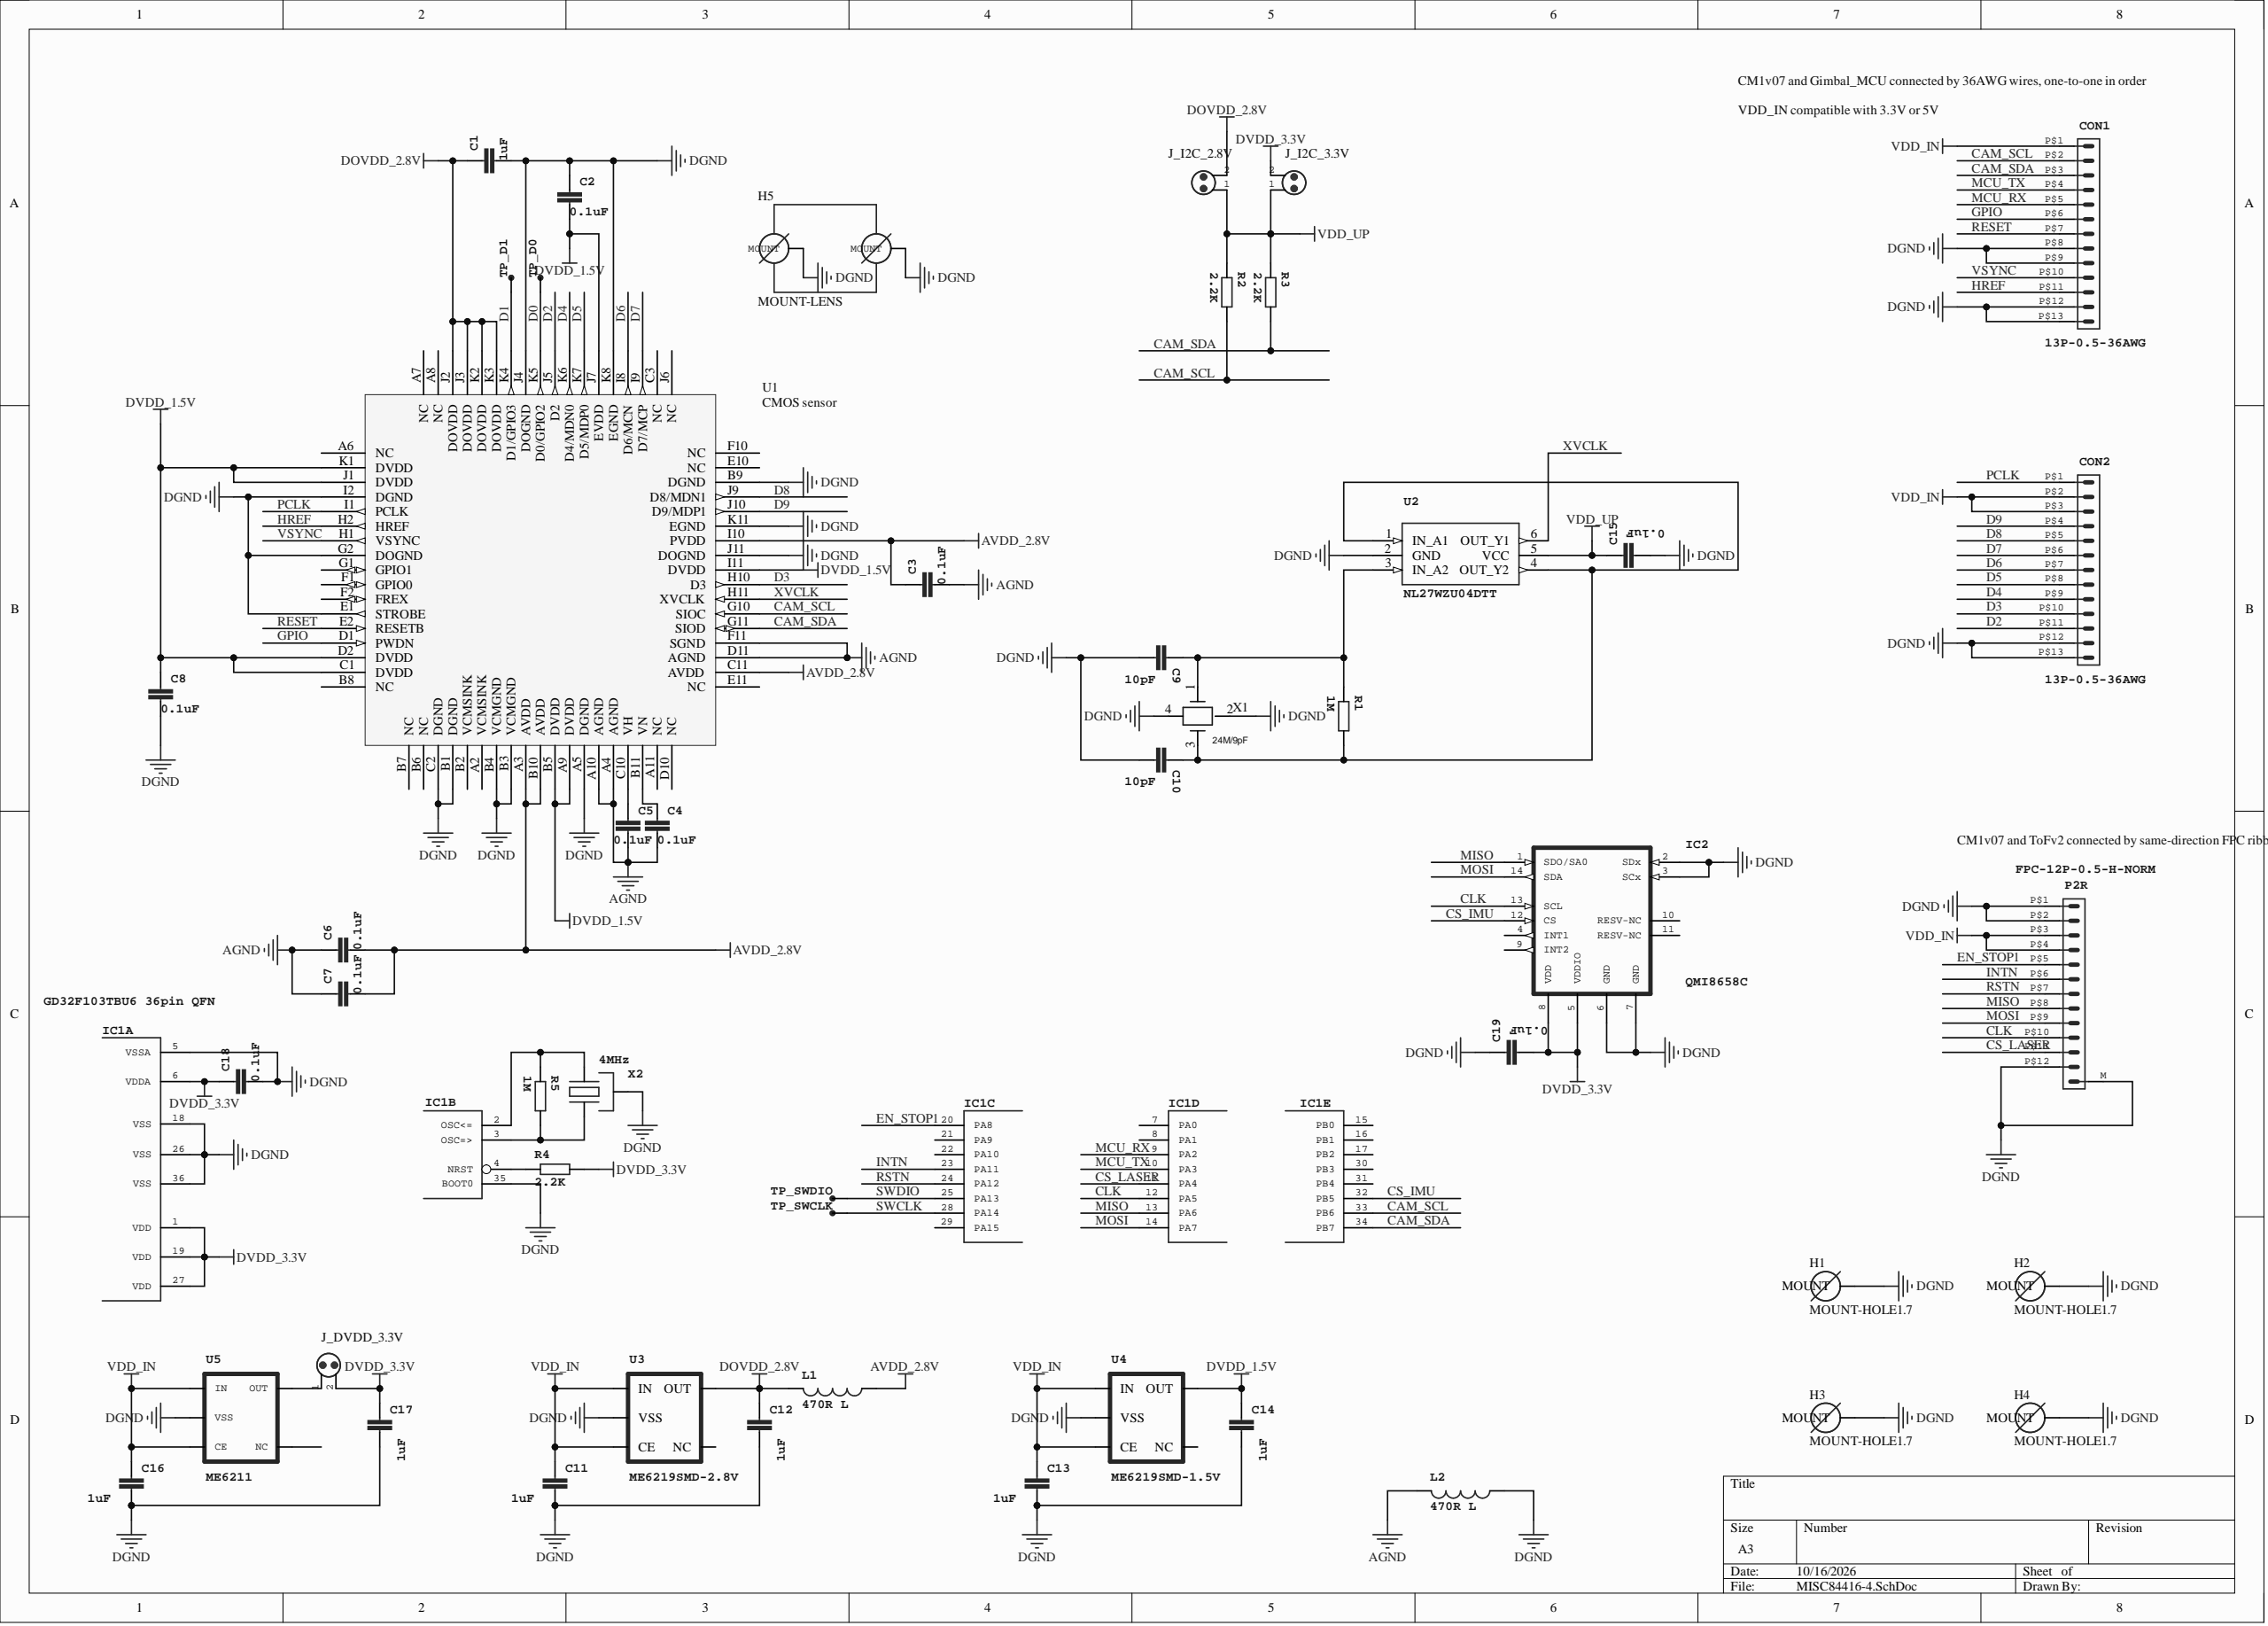Circuit board | Altium Designer | 50 parts | 46 nets
Bill of materials:
Comment,Description,Designator,Footprint,LibRef,Quantity
"1uF","","C1, C11, C12, C13, C14, C16, C17","RCL_C0402_TI","RCL_C-EUC0402_TI","7"
"0.1uF","","C2, C3, C4, C5, C6, C7, C8, C15, C18, C19","RCL_C0402_TI","RCL_C-EUC0402_TI","10"
"10pF","","C9, C10","RCL_C0402_TI","RCL_C-EUC0402_TI","2"
"13P-0.5-36AWG","","CON1, CON2","13P-0.5-36AWG","13P-0.5-36AWG","2"
"MOUNT-HOLE1.7","","H1, H2, H3, H4","MOUNT-HOLE1.7","MOUNT-HOLE1.7","4"
"MOUNT-LENS","","H5","MOUNT-LENS-M12-1.6","MOUNT-LENS","1"
"GD32F103TBU6 36pin QFN","","IC1","GD32_QFN36","GD32F103TBU6","1"
"QMI8658C","","IC2","LGA14_3X2.5","QMI8658C","1"
"JUMPER_2P_MIN","","J_DVDD_3.3V, J_I2C_2.8V, J_I2C_3.3V","JUMPER_2P_MIN","JUMPER_2P_MIN","3"
"470R L","","L1, L2","RCL_L0603","RCL_L-USL0603","2"
"FPC-12P-0.5-H-NORM","","P2R","FPC-12P-0.5-H-NORM","FPC-12P-0.5-H-NORM","1"
"1M","","R1, R5","RCL_R0402_TI","RCL_R-EUR0402_TI","2"
"2.2K","","R2, R3, R4","RCL_R0402_TI","RCL_R-EUR0402_TI","3"
"","","TP_D0, TP_D1, TP_SWCLK, TP_SWDIO","TP-1","TP-1","4"
"CMOS sensor","1/4INCH","U1","BGA71_5.99X5.84","OV5640","1"
"NL27WZU04DTT","","U2","SOT23-6","NL27WZU04DTT","1"
"ME6219SMD-2.8V","","U3","SOT23-5","ME6219SMD","1"
"ME6219SMD-1.5V","","U4","SOT23-5","ME6219SMD","1"
"ME6211","","U5","SOT23-5","ME6211SMD","1"
"24M/9pF","","X1","EPSON-TSX3225","XTAL_EPSON_3225","1"
"4MHz","","X2","XTAL_4.5X2.0","XTAL_MURATA-4.5X2.0","1"
Netlist (Protel format):
[
C1
RCL_C0402_TI
1uF



]
[
C2
RCL_C0402_TI
0.1uF



]
[
C3
RCL_C0402_TI
0.1uF



]
[
C4
RCL_C0402_TI
0.1uF



]
[
C5
RCL_C0402_TI
0.1uF



]
[
C6
RCL_C0402_TI
0.1uF



]
[
C7
RCL_C0402_TI
0.1uF



]
[
C8
RCL_C0402_TI
0.1uF



]
[
C9
RCL_C0402_TI
10pF



]
[
C10
RCL_C0402_TI
10pF



]
[
C11
RCL_C0402_TI
1uF



]
[
C12
RCL_C0402_TI
1uF



]
[
C13
RCL_C0402_TI
1uF



]
[
C14
RCL_C0402_TI
1uF



]
[
C15
RCL_C0402_TI
0.1uF



]
[
C16
RCL_C0402_TI
1uF



]
[
C17
RCL_C0402_TI
1uF



]
[
C18
RCL_C0402_TI
0.1uF



]
[
C19
RCL_C0402_TI
0.1uF



]
[
CON1
13P-0.5-36AWG
13P-0.5-36AWG



]
[
CON2
13P-0.5-36AWG
13P-0.5-36AWG



]
[
H1
MOUNT-HOLE1.7
MOUNT-HOLE1.7



]
[
H2
MOUNT-HOLE1.7
MOUNT-HOLE1.7



]
[
H3
MOUNT-HOLE1.7
MOUNT-HOLE1.7



]
[
H4
MOUNT-HOLE1.7
MOUNT-HOLE1.7



]
[
H5
MOUNT-LENS-M12-1.6
MOUNT-LENS



]
[
IC1
GD32_QFN36
GD32F103TBU6 36pin QFN



]
[
IC2
LGA14_3X2.5
QMI8658C



]
[
J_DVDD_3.3V
JUMPER_2P_MIN
JUMPER_2P_MIN



]
[
J_I2C_2.8V
JUMPER_2P_MIN
JUMPER_2P_MIN



]
[
J_I2C_3.3V
JUMPER_2P_MIN
JUMPER_2P_MIN



]
[
L1
RCL_L0603
470R L



]
[
L2
RCL_L0603
470R L



]
[
P2R
FPC-12P-0.5-H-NORM
FPC-12P-0.5-H-NORM



]
[
R1
RCL_R0402_TI
1M



]
[
R2
RCL_R0402_TI
2.2K



]
[
R3
RCL_R0402_TI
2.2K



]
[
R4
RCL_R0402_TI
2.2K



]
[
R5
RCL_R0402_TI
1M



]
[
TP_D0
TP-1




]
[
TP_D1
TP-1




]
[
TP_SWCLK
TP-1




]
[
TP_SWDIO
TP-1




]
[
U1
BGA71_5.99X5.84
CMOS sensor



]
[
U2
SOT23-6
NL27WZU04DTT



]
[
U3
SOT23-5
ME6219SMD-2.8V



]
[
U4
SOT23-5
ME6219SMD-1.5V



]
[
U5
SOT23-5
ME6211



]
[
X1
EPSON-TSX3225
24M/9pF



]
[
X2
XTAL_4.5X2.0
4MHz



]
(
XVCLK
U1-H11
U2-6
)
(
VSYNC
CON1-P$10
U1-H1
)
(
VDD_UP
C15-1
J_I2C_2.8V-1
J_I2C_3.3V-1
R2-1
R3-1
U2-5
)
(
VDD_IN
C11-1
C13-1
C16-1
CON1-P$1
CON2-P$2
CON2-P$3
P2R-P$3
P2R-P$4
U3-1
U3-3
U4-1
U4-3
U5-1
U5-3
)
(
SWDIO
IC1-25
TP_SWDIO-1
)
(
SWCLK
IC1-28
TP_SWCLK-1
)
(
RSTN
IC1-24
P2R-P$7
)
(
RESET
CON1-P$7
U1-E2
)
(
PCLK
CON2-P$1
U1-I1
)
(
NetJ_DVDD_3.3V_1
J_DVDD_3.3V-1
U5-5
)
(
NetIC1_4
IC1-4
R4-1
)
(
NetIC1_3
IC1-3
R5-2
X2-1
)
(
NetIC1_2
IC1-2
R5-1
X2-3
)
(
NetC10_1
C10-1
R1-2
U2-1
U2-4
X1-3
)
(
NetC9_1
C9-1
R1-1
U2-3
X1-1
)
(
NetC5_1
C5-1
U1-C10
)
(
NetC4_1
C4-1
U1-B11
)
(
MOSI
IC1-14
IC2-14
P2R-P$9
)
(
MISO
IC1-13
IC2-1
P2R-P$8
)
(
MCU_TX
CON1-P$4
IC1-10
)
(
MCU_RX
CON1-P$5
IC1-9
)
(
INTN
IC1-23
P2R-P$6
)
(
HREF
CON1-P$11
U1-H2
)
(
GPIO
CON1-P$6
U1-D1
)
(
EN_STOP1
IC1-20
P2R-P$5
)
(
DVDD_3.3V
C17-1
C18-1
C19-2
IC1-1
IC1-6
IC1-19
IC1-27
IC2-5
IC2-8
J_DVDD_3.3V-2
J_I2C_3.3V-2
R4-2
)
(
DVDD_1.5V
C2-2
C8-1
C14-1
U1-A9
U1-B5
U1-C1
U1-D2
U1-I11
U1-J1
U1-J7
U1-K1
U4-5
)
(
DOVDD_2.8V
C1-1
C12-1
J_I2C_2.8V-2
L1-2
U1-J2
U1-J3
U1-K2
U1-K3
U3-5
)
(
DGND
C1-2
C2-1
C8-2
C9-2
C10-2
C11-2
C12-2
C13-2
C14-2
C15-2
C16-2
C17-2
C18-2
C19-1
CON1-P$8
CON1-P$9
CON1-P$12
CON1-P$13
CON2-P$12
CON2-P$13
H1-MOUNT
H2-MOUNT
H3-MOUNT
H4-MOUNT
H5-MOUNT
IC1-5
IC1-18
IC1-26
IC1-35
IC1-36
IC2-2
IC2-3
IC2-6
IC2-7
L2-1
P2R-M
P2R-P$1
P2R-P$2
P2R-P$12
U1-A5
U1-B1
U1-B3
U1-B4
U1-B9
U1-C2
U1-E1
U1-G2
U1-I2
U1-J4
U1-J11
U1-K8
U1-K11
U2-2
U3-2
U4-2
U5-2
X1-2
X1-4
X2-2
)
(
D9
CON2-P$4
U1-J10
)
(
D8
CON2-P$5
U1-J9
)
(
D7
CON2-P$6
U1-I9
)
(
D6
CON2-P$7
U1-I8
)
(
D5
CON2-P$8
U1-K7
)
(
D4
CON2-P$9
U1-K6
)
(
D3
CON2-P$10
U1-H10
)
(
D2
CON2-P$11
U1-J5
)
(
D1
TP_D1-1
U1-K4
)
(
D0
TP_D0-1
U1-K5
)
(
CS_LASER
IC1-11
P2R-P$11
)
(
CS_IMU
IC1-32
IC2-12
)
(
CLK
IC1-12
IC2-13
P2R-P$10
)
(
CAM_SDA
CON1-P$3
IC1-34
R3-2
U1-G11
)
(
CAM_SCL
CON1-P$2
IC1-33
R2-2
U1-G10
)
(
AVDD_2.8V
C3-1
C6-2
C7-2
L1-1
U1-A3
U1-B10
U1-C11
U1-I10
)
(
AGND
C3-2
C4-2
C5-2
C6-1
C7-1
L2-2
U1-A4
U1-A10
U1-D11
U1-F11
)